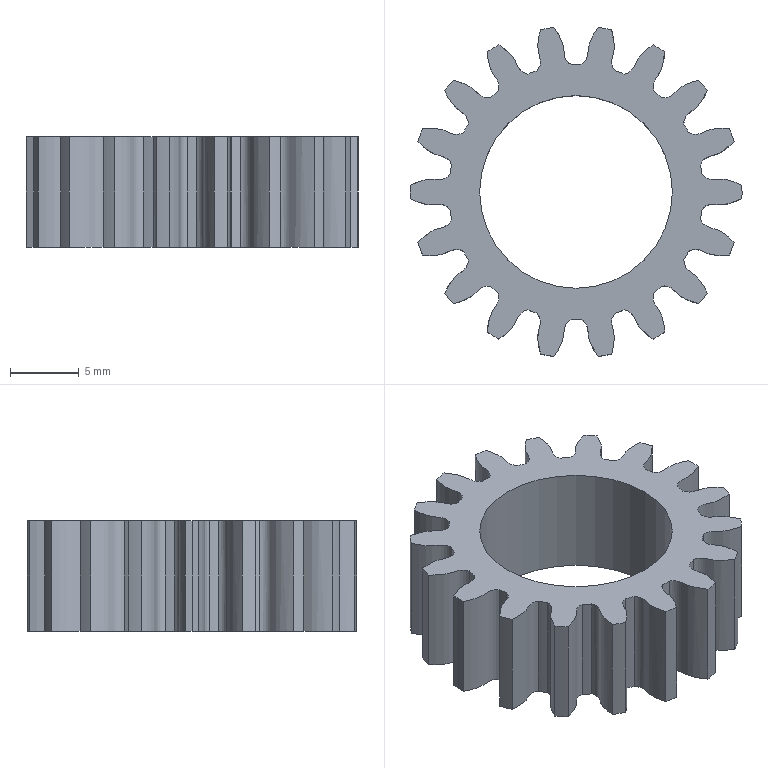Part | SolidWorks | features ICE 2, CirPattern 1, Extrusion 1, RefAxis 1 | 1 solid | 77 faces | box 24.125 x 23.91 x 8 mm | volume 1615 mm3 | cylinder 39 | spline 36 | plane 2 | commonest cylinder face diameters 24.125 x19 18.5 x18 14 x2